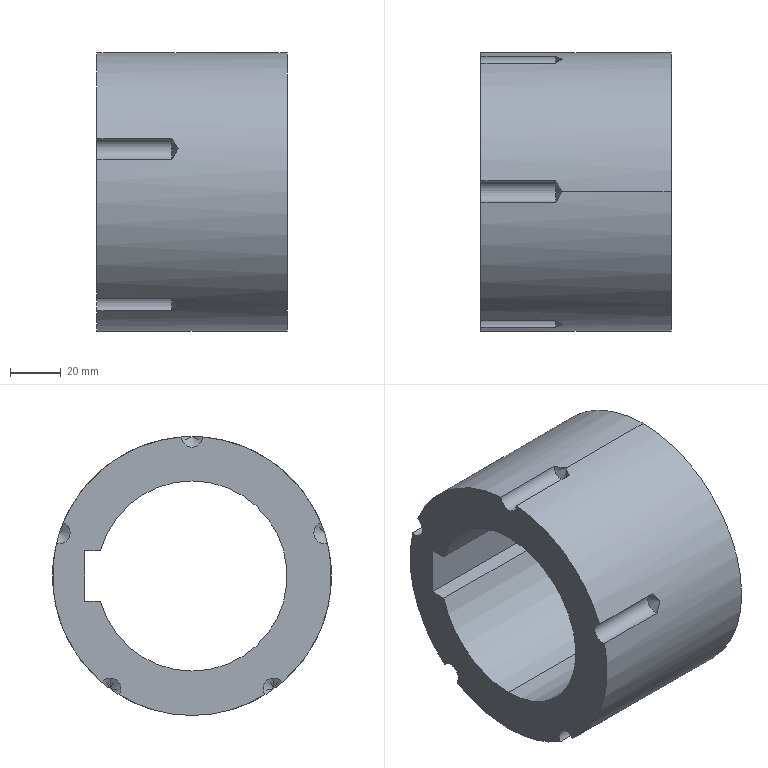Part | SolidWorks | features HoleWzd 1, ICE 1, Revolution 1 | 1 solid | 24 faces | box 75 x 110 x 110 mm | volume 369149 mm3 | cylinder 12 | cone 7 | plane 5 | commonest cylinder face diameters 8.5 x7 75 x3 110 x2
STEP:
#1=CARTESIAN_POINT('',(32.054,-32.328,-44.496));
#2=VERTEX_POINT('',#1);
#3=CARTESIAN_POINT('',(29.5,-28.796,-46.859));
#4=VERTEX_POINT('',#3);
#5=CARTESIAN_POINT('',(32.054,-32.328,-44.496));
#6=CARTESIAN_POINT('',(31.202,-31.182,-45.329));
#7=CARTESIAN_POINT('',(30.351,-30.003,-46.118));
#8=CARTESIAN_POINT('',(29.5,-28.796,-46.859));
#9=B_SPLINE_CURVE_WITH_KNOTS('',3,(#5,#6,#7,#8),.UNSPECIFIED.,.F.,.F.,(4,4),(-0.000000022,0.00496),.UNSPECIFIED.);
#10=EDGE_CURVE('',#2,#4,#9,.T.);
#11=ORIENTED_EDGE('',*,*,#10,.F.);
#12=CARTESIAN_POINT('',(29.5,-32.328,-40.246));
#13=VERTEX_POINT('',#12);
#14=CARTESIAN_POINT('',(29.5,-32.328,-40.246));
#15=DIRECTION('',(-0.515,0.,0.8572));
#16=VECTOR('',#15,1000.);
#17=LINE('',#14,#16);
#18=EDGE_CURVE('',#2,#13,#17,.T.);
#19=ORIENTED_EDGE('',*,*,#18,.T.);
#20=CARTESIAN_POINT('',(29.5,-32.328,-44.496));
#21=DIRECTION('',(-1.,0.,0.));
#22=DIRECTION('',(0.,0.,1.));
#23=AXIS2_PLACEMENT_3D('',#20,#21,#22);
#24=CIRCLE('',#23,4.25);
#25=EDGE_CURVE('',#13,#4,#24,.T.);
#26=ORIENTED_EDGE('',*,*,#25,.T.);
#27=EDGE_LOOP('',(#11,#19,#26));
#28=FACE_OUTER_BOUND('',#27,.T.);
#29=CARTESIAN_POINT('',(29.5,-32.328,-44.496));
#30=DIRECTION('',(-1.,0.,0.));
#31=DIRECTION('',(0.,0.,1.));
#32=AXIS2_PLACEMENT_3D('',#29,#30,#31);
#33=CONICAL_SURFACE('',#32,4.25,1.03);
#34=ADVANCED_FACE('',(#28),#33,.F.);
#35=ORIENTED_EDGE('',*,*,#25,.F.);
#36=CARTESIAN_POINT('',(0.,-32.328,-40.246));
#37=VERTEX_POINT('',#36);
#38=CARTESIAN_POINT('',(0.,-32.328,-40.246));
#39=DIRECTION('',(-1.,0.,0.));
#40=VECTOR('',#39,1000.);
#41=LINE('',#38,#40);
#42=EDGE_CURVE('',#13,#37,#41,.T.);
#43=ORIENTED_EDGE('',*,*,#42,.T.);
#44=CARTESIAN_POINT('',(0.,-28.796,-46.859));
#45=VERTEX_POINT('',#44);
#46=CARTESIAN_POINT('',(0.,-32.328,-44.496));
#47=DIRECTION('',(-1.,0.,0.));
#48=DIRECTION('',(0.,0.,1.));
#49=AXIS2_PLACEMENT_3D('',#46,#47,#48);
#50=CIRCLE('',#49,4.25);
#51=EDGE_CURVE('',#37,#45,#50,.T.);
#52=ORIENTED_EDGE('',*,*,#51,.T.);
#53=CARTESIAN_POINT('',(14.75,-28.796,-46.859));
#54=DIRECTION('',(-1.,0.,0.));
#55=VECTOR('',#54,1000.);
#56=LINE('',#53,#55);
#57=EDGE_CURVE('',#4,#45,#56,.T.);
#58=ORIENTED_EDGE('',*,*,#57,.F.);
#59=EDGE_LOOP('',(#35,#43,#52,#58));
#60=FACE_OUTER_BOUND('',#59,.T.);
#61=CARTESIAN_POINT('',(0.,-32.328,-44.496));
#62=DIRECTION('',(-1.,0.,0.));
#63=DIRECTION('',(0.,0.,1.));
#64=AXIS2_PLACEMENT_3D('',#61,#62,#63);
#65=CYLINDRICAL_SURFACE('',#64,4.25);
#66=ADVANCED_FACE('',(#60),#65,.F.);
#67=CARTESIAN_POINT('',(32.054,32.328,-44.496));
#68=VERTEX_POINT('',#67);
#69=CARTESIAN_POINT('',(29.5,35.667,-41.867));
#70=VERTEX_POINT('',#69);
#71=CARTESIAN_POINT('',(32.054,32.328,-44.496));
#72=CARTESIAN_POINT('',(31.202,33.475,-43.663));
#73=CARTESIAN_POINT('',(30.351,34.589,-42.785));
#74=CARTESIAN_POINT('',(29.5,35.667,-41.867));
#75=B_SPLINE_CURVE_WITH_KNOTS('',3,(#71,#72,#73,#74),.UNSPECIFIED.,.F.,.F.,(4,4),(-0.000000022,0.00496),.UNSPECIFIED.);
#76=EDGE_CURVE('',#68,#70,#75,.T.);
#77=ORIENTED_EDGE('',*,*,#76,.F.);
#78=CARTESIAN_POINT('',(29.5,32.328,-40.246));
#79=VERTEX_POINT('',#78);
#80=CARTESIAN_POINT('',(29.5,32.328,-40.246));
#81=DIRECTION('',(-0.515,0.,0.8572));
#82=VECTOR('',#81,1000.);
#83=LINE('',#80,#82);
#84=EDGE_CURVE('',#68,#79,#83,.T.);
#85=ORIENTED_EDGE('',*,*,#84,.T.);
#86=CARTESIAN_POINT('',(29.5,32.328,-44.496));
#87=DIRECTION('',(-1.,0.,0.));
#88=DIRECTION('',(0.,0.,1.));
#89=AXIS2_PLACEMENT_3D('',#86,#87,#88);
#90=CIRCLE('',#89,4.25);
#91=EDGE_CURVE('',#79,#70,#90,.T.);
#92=ORIENTED_EDGE('',*,*,#91,.T.);
#93=EDGE_LOOP('',(#77,#85,#92));
#94=FACE_OUTER_BOUND('',#93,.T.);
#95=CARTESIAN_POINT('',(29.5,32.328,-44.496));
#96=DIRECTION('',(-1.,0.,0.));
#97=DIRECTION('',(0.,0.,1.));
#98=AXIS2_PLACEMENT_3D('',#95,#96,#97);
#99=CONICAL_SURFACE('',#98,4.25,1.03);
#100=ADVANCED_FACE('',(#94),#99,.F.);
#101=ORIENTED_EDGE('',*,*,#91,.F.);
#102=CARTESIAN_POINT('',(0.,32.328,-40.246));
#103=VERTEX_POINT('',#102);
#104=CARTESIAN_POINT('',(0.,32.328,-40.246));
#105=DIRECTION('',(-1.,0.,0.));
#106=VECTOR('',#105,1000.);
#107=LINE('',#104,#106);
#108=EDGE_CURVE('',#79,#103,#107,.T.);
#109=ORIENTED_EDGE('',*,*,#108,.T.);
#110=CARTESIAN_POINT('',(0.,35.667,-41.867));
#111=VERTEX_POINT('',#110);
#112=CARTESIAN_POINT('',(0.,32.328,-44.496));
#113=DIRECTION('',(-1.,0.,0.));
#114=DIRECTION('',(0.,0.,1.));
#115=AXIS2_PLACEMENT_3D('',#112,#113,#114);
#116=CIRCLE('',#115,4.25);
#117=EDGE_CURVE('',#103,#111,#116,.T.);
#118=ORIENTED_EDGE('',*,*,#117,.T.);
#119=CARTESIAN_POINT('',(14.75,35.667,-41.867));
#120=DIRECTION('',(-1.,0.,0.));
#121=VECTOR('',#120,1000.);
#122=LINE('',#119,#121);
#123=EDGE_CURVE('',#70,#111,#122,.T.);
#124=ORIENTED_EDGE('',*,*,#123,.F.);
#125=EDGE_LOOP('',(#101,#109,#118,#124));
#126=FACE_OUTER_BOUND('',#125,.T.);
#127=CARTESIAN_POINT('',(0.,32.328,-44.496));
#128=DIRECTION('',(-1.,0.,0.));
#129=DIRECTION('',(0.,0.,1.));
#130=AXIS2_PLACEMENT_3D('',#127,#128,#129);
#131=CYLINDRICAL_SURFACE('',#130,4.25);
#132=ADVANCED_FACE('',(#126),#131,.F.);
#133=CARTESIAN_POINT('',(75.,0.,55.));
#134=VERTEX_POINT('',#133);
#135=CARTESIAN_POINT('',(75.,0.,-55.));
#136=VERTEX_POINT('',#135);
#137=CARTESIAN_POINT('',(75.,0.,0.));
#138=DIRECTION('',(-1.,0.,0.));
#139=DIRECTION('',(0.,0.,1.));
#140=AXIS2_PLACEMENT_3D('',#137,#138,#139);
#141=CIRCLE('',#140,55.);
#142=EDGE_CURVE('',#134,#136,#141,.T.);
#143=ORIENTED_EDGE('',*,*,#142,.T.);
#144=CARTESIAN_POINT('',(0.,0.,-55.));
#145=VERTEX_POINT('',#144);
#146=CARTESIAN_POINT('',(0.,0.,-55.));
#147=DIRECTION('',(-1.,0.,0.));
#148=VECTOR('',#147,1000.);
#149=LINE('',#146,#148);
#150=EDGE_CURVE('',#136,#145,#149,.T.);
#151=ORIENTED_EDGE('',*,*,#150,.T.);
#152=CARTESIAN_POINT('',(0.,28.796,-46.859));
#153=VERTEX_POINT('',#152);
#154=CARTESIAN_POINT('',(0.,0.,0.));
#155=DIRECTION('',(-1.,0.,0.));
#156=DIRECTION('',(0.,0.,1.));
#157=AXIS2_PLACEMENT_3D('',#154,#155,#156);
#158=CIRCLE('',#157,55.);
#159=EDGE_CURVE('',#153,#145,#158,.T.);
#160=ORIENTED_EDGE('',*,*,#159,.F.);
#161=CARTESIAN_POINT('',(29.5,28.796,-46.859));
#162=VERTEX_POINT('',#161);
#163=CARTESIAN_POINT('',(14.75,28.796,-46.859));
#164=DIRECTION('',(1.,0.,0.));
#165=VECTOR('',#164,1000.);
#166=LINE('',#163,#165);
#167=EDGE_CURVE('',#153,#162,#166,.T.);
#168=ORIENTED_EDGE('',*,*,#167,.T.);
#169=CARTESIAN_POINT('',(29.5,28.796,-46.859));
#170=CARTESIAN_POINT('',(29.925,29.399,-46.488));
#171=CARTESIAN_POINT('',(30.351,29.996,-46.106));
#172=CARTESIAN_POINT('',(30.989,30.879,-45.515));
#173=CARTESIAN_POINT('',(31.202,31.172,-45.315));
#174=CARTESIAN_POINT('',(31.628,31.753,-44.91));
#175=CARTESIAN_POINT('',(31.842,32.043,-44.703));
#176=CARTESIAN_POINT('',(32.054,32.328,-44.496));
#177=B_SPLINE_CURVE_WITH_KNOTS('',3,(#169,#170,#171,#172,#173,#174,#175,#176),.UNSPECIFIED.,.F.,.F.,(4,2,2,4),(0.01174,0.01422,0.01545,0.01669),.UNSPECIFIED.);
#178=EDGE_CURVE('',#162,#68,#177,.T.);
#179=ORIENTED_EDGE('',*,*,#178,.T.);
#180=ORIENTED_EDGE('',*,*,#76,.T.);
#181=ORIENTED_EDGE('',*,*,#123,.T.);
#182=CARTESIAN_POINT('',(0.,53.464,12.906));
#183=VERTEX_POINT('',#182);
#184=CARTESIAN_POINT('',(0.,0.,0.));
#185=DIRECTION('',(-1.,0.,0.));
#186=DIRECTION('',(0.,0.,1.));
#187=AXIS2_PLACEMENT_3D('',#184,#185,#186);
#188=CIRCLE('',#187,55.);
#189=EDGE_CURVE('',#183,#111,#188,.T.);
#190=ORIENTED_EDGE('',*,*,#189,.F.);
#191=CARTESIAN_POINT('',(29.5,53.464,12.906));
#192=VERTEX_POINT('',#191);
#193=CARTESIAN_POINT('',(14.75,53.464,12.906));
#194=DIRECTION('',(1.,0.,0.));
#195=VECTOR('',#194,1000.);
#196=LINE('',#193,#195);
#197=EDGE_CURVE('',#183,#192,#196,.T.);
#198=ORIENTED_EDGE('',*,*,#197,.T.);
#199=CARTESIAN_POINT('',(32.054,52.308,16.996));
#200=VERTEX_POINT('',#199);
#201=CARTESIAN_POINT('',(29.5,53.464,12.906));
#202=CARTESIAN_POINT('',(29.925,53.298,13.595));
#203=CARTESIAN_POINT('',(30.351,53.118,14.281));
#204=CARTESIAN_POINT('',(30.989,52.829,15.303));
#205=CARTESIAN_POINT('',(31.202,52.73,15.643));
#206=CARTESIAN_POINT('',(31.628,52.524,16.321));
#207=CARTESIAN_POINT('',(31.841,52.417,16.66));
#208=CARTESIAN_POINT('',(32.054,52.308,16.996));
#209=B_SPLINE_CURVE_WITH_KNOTS('',3,(#201,#202,#203,#204,#205,#206,#207,#208),.UNSPECIFIED.,.F.,.F.,(4,2,2,4),(0.01071,0.01319,0.01442,0.01566),.UNSPECIFIED.);
#210=EDGE_CURVE('',#192,#200,#209,.T.);
#211=ORIENTED_EDGE('',*,*,#210,.T.);
#212=CARTESIAN_POINT('',(29.5,50.84,20.984));
#213=VERTEX_POINT('',#212);
#214=CARTESIAN_POINT('',(32.054,52.308,16.996));
#215=CARTESIAN_POINT('',(31.202,51.87,18.344));
#216=CARTESIAN_POINT('',(30.351,51.38,19.675));
#217=CARTESIAN_POINT('',(29.5,50.84,20.984));
#218=B_SPLINE_CURVE_WITH_KNOTS('',3,(#214,#215,#216,#217),.UNSPECIFIED.,.F.,.F.,(4,4),(-0.000000022,0.00496),.UNSPECIFIED.);
#219=EDGE_CURVE('',#200,#213,#218,.T.);
#220=ORIENTED_EDGE('',*,*,#219,.T.);
#221=CARTESIAN_POINT('',(0.,50.84,20.984));
#222=VERTEX_POINT('',#221);
#223=CARTESIAN_POINT('',(14.75,50.84,20.984));
#224=DIRECTION('',(-1.,0.,0.));
#225=VECTOR('',#224,1000.);
#226=LINE('',#223,#225);
#227=EDGE_CURVE('',#213,#222,#226,.T.);
#228=ORIENTED_EDGE('',*,*,#227,.T.);
#229=CARTESIAN_POINT('',(0.,4.247,54.836));
#230=VERTEX_POINT('',#229);
#231=CARTESIAN_POINT('',(0.,0.,0.));
#232=DIRECTION('',(-1.,0.,0.));
#233=DIRECTION('',(0.,0.,1.));
#234=AXIS2_PLACEMENT_3D('',#231,#232,#233);
#235=CIRCLE('',#234,55.);
#236=EDGE_CURVE('',#230,#222,#235,.T.);
#237=ORIENTED_EDGE('',*,*,#236,.F.);
#238=CARTESIAN_POINT('',(29.5,4.247,54.836));
#239=VERTEX_POINT('',#238);
#240=CARTESIAN_POINT('',(14.75,4.247,54.836));
#241=DIRECTION('',(1.,0.,0.));
#242=VECTOR('',#241,1000.);
#243=LINE('',#240,#242);
#244=EDGE_CURVE('',#230,#239,#243,.T.);
#245=ORIENTED_EDGE('',*,*,#244,.T.);
#246=CARTESIAN_POINT('',(32.054,0.,55.));
#247=VERTEX_POINT('',#246);
#248=CARTESIAN_POINT('',(29.5,4.247,54.836));
#249=CARTESIAN_POINT('',(29.925,3.541,54.89));
#250=CARTESIAN_POINT('',(30.351,2.833,54.932));
#251=CARTESIAN_POINT('',(31.202,1.417,54.986));
#252=CARTESIAN_POINT('',(31.629,0.707,55.));
#253=CARTESIAN_POINT('',(32.054,0.,55.));
#254=B_SPLINE_CURVE_WITH_KNOTS('',3,(#248,#249,#250,#251,#252,#253),.UNSPECIFIED.,.F.,.F.,(4,2,4),(0.009274,0.01175,0.01422),.UNSPECIFIED.);
#255=EDGE_CURVE('',#239,#247,#254,.T.);
#256=ORIENTED_EDGE('',*,*,#255,.T.);
#257=CARTESIAN_POINT('',(0.,0.,55.));
#258=DIRECTION('',(-1.,0.,0.));
#259=VECTOR('',#258,1000.);
#260=LINE('',#257,#259);
#261=EDGE_CURVE('',#134,#247,#260,.T.);
#262=ORIENTED_EDGE('',*,*,#261,.F.);
#263=EDGE_LOOP('',(#143,#151,#160,#168,#179,#180,#181,#190,#198,#211,#220,#228,#237,#245,#256,#262));
#264=FACE_OUTER_BOUND('',#263,.T.);
#265=CARTESIAN_POINT('',(0.,0.,0.));
#266=DIRECTION('',(-1.,0.,0.));
#267=DIRECTION('',(0.,0.,1.));
#268=AXIS2_PLACEMENT_3D('',#265,#266,#267);
#269=CYLINDRICAL_SURFACE('',#268,55.);
#270=ADVANCED_FACE('',(#264),#269,.T.);
#271=CARTESIAN_POINT('',(75.,0.,-37.5));
#272=VERTEX_POINT('',#271);
#273=CARTESIAN_POINT('',(75.,0.,37.5));
#274=VERTEX_POINT('',#273);
#275=CARTESIAN_POINT('',(75.,0.,0.));
#276=DIRECTION('',(-1.,0.,0.));
#277=DIRECTION('',(0.,0.,1.));
#278=AXIS2_PLACEMENT_3D('',#275,#276,#277);
#279=CIRCLE('',#278,37.5);
#280=EDGE_CURVE('',#272,#274,#279,.T.);
#281=ORIENTED_EDGE('',*,*,#280,.F.);
#282=CARTESIAN_POINT('',(0.,0.,-37.5));
#283=VERTEX_POINT('',#282);
#284=CARTESIAN_POINT('',(0.,0.,-37.5));
#285=DIRECTION('',(-1.,0.,0.));
#286=VECTOR('',#285,1000.);
#287=LINE('',#284,#286);
#288=EDGE_CURVE('',#272,#283,#287,.T.);
#289=ORIENTED_EDGE('',*,*,#288,.T.);
#290=CARTESIAN_POINT('',(0.,0.,37.5));
#291=VERTEX_POINT('',#290);
#292=CARTESIAN_POINT('',(0.,0.,0.));
#293=DIRECTION('',(-1.,0.,0.));
#294=DIRECTION('',(0.,0.,1.));
#295=AXIS2_PLACEMENT_3D('',#292,#293,#294);
#296=CIRCLE('',#295,37.5);
#297=EDGE_CURVE('',#283,#291,#296,.T.);
#298=ORIENTED_EDGE('',*,*,#297,.T.);
#299=CARTESIAN_POINT('',(0.,0.,37.5));
#300=DIRECTION('',(-1.,0.,0.));
#301=VECTOR('',#300,1000.);
#302=LINE('',#299,#301);
#303=EDGE_CURVE('',#274,#291,#302,.T.);
#304=ORIENTED_EDGE('',*,*,#303,.F.);
#305=EDGE_LOOP('',(#281,#289,#298,#304));
#306=FACE_OUTER_BOUND('',#305,.T.);
#307=CARTESIAN_POINT('',(0.,0.,0.));
#308=DIRECTION('',(-1.,0.,0.));
#309=DIRECTION('',(0.,0.,1.));
#310=AXIS2_PLACEMENT_3D('',#307,#308,#309);
#311=CYLINDRICAL_SURFACE('',#310,37.5);
#312=ADVANCED_FACE('',(#306),#311,.F.);
#313=CARTESIAN_POINT('',(75.,36.142,10.));
#314=VERTEX_POINT('',#313);
#315=CARTESIAN_POINT('',(75.,0.,0.));
#316=DIRECTION('',(-1.,0.,0.));
#317=DIRECTION('',(0.,0.,1.));
#318=AXIS2_PLACEMENT_3D('',#315,#316,#317);
#319=CIRCLE('',#318,37.5);
#320=EDGE_CURVE('',#274,#314,#319,.T.);
#321=ORIENTED_EDGE('',*,*,#320,.F.);
#322=ORIENTED_EDGE('',*,*,#303,.T.);
#323=CARTESIAN_POINT('',(0.,36.142,10.));
#324=VERTEX_POINT('',#323);
#325=CARTESIAN_POINT('',(0.,0.,0.));
#326=DIRECTION('',(-1.,0.,0.));
#327=DIRECTION('',(0.,0.,1.));
#328=AXIS2_PLACEMENT_3D('',#325,#326,#327);
#329=CIRCLE('',#328,37.5);
#330=EDGE_CURVE('',#291,#324,#329,.T.);
#331=ORIENTED_EDGE('',*,*,#330,.T.);
#332=CARTESIAN_POINT('',(0.,36.142,10.));
#333=DIRECTION('',(-1.,0.,0.));
#334=VECTOR('',#333,1000.);
#335=LINE('',#332,#334);
#336=EDGE_CURVE('',#314,#324,#335,.T.);
#337=ORIENTED_EDGE('',*,*,#336,.F.);
#338=EDGE_LOOP('',(#321,#322,#331,#337));
#339=FACE_OUTER_BOUND('',#338,.T.);
#340=CARTESIAN_POINT('',(0.,0.,0.));
#341=DIRECTION('',(-1.,0.,0.));
#342=DIRECTION('',(0.,0.,1.));
#343=AXIS2_PLACEMENT_3D('',#340,#341,#342);
#344=CYLINDRICAL_SURFACE('',#343,37.5);
#345=ADVANCED_FACE('',(#339),#344,.F.);
#346=CARTESIAN_POINT('',(0.,36.142,-10.));
#347=VERTEX_POINT('',#346);
#348=CARTESIAN_POINT('',(0.,0.,0.));
#349=DIRECTION('',(-1.,0.,0.));
#350=DIRECTION('',(0.,0.,1.));
#351=AXIS2_PLACEMENT_3D('',#348,#349,#350);
#352=CIRCLE('',#351,37.5);
#353=EDGE_CURVE('',#347,#283,#352,.T.);
#354=ORIENTED_EDGE('',*,*,#353,.F.);
#355=CARTESIAN_POINT('',(0.,42.4,-10.));
#356=VERTEX_POINT('',#355);
#357=CARTESIAN_POINT('',(0.,-55.001,-10.));
#358=DIRECTION('',(0.,1.,0.));
#359=VECTOR('',#358,1000.);
#360=LINE('',#357,#359);
#361=EDGE_CURVE('',#347,#356,#360,.T.);
#362=ORIENTED_EDGE('',*,*,#361,.T.);
#363=CARTESIAN_POINT('',(0.,42.4,10.));
#364=VERTEX_POINT('',#363);
#365=CARTESIAN_POINT('',(0.,42.4,-10.));
#366=DIRECTION('',(0.,0.,1.));
#367=VECTOR('',#366,1000.);
#368=LINE('',#365,#367);
#369=EDGE_CURVE('',#356,#364,#368,.T.);
#370=ORIENTED_EDGE('',*,*,#369,.T.);
#371=CARTESIAN_POINT('',(0.,-55.001,10.));
#372=DIRECTION('',(0.,1.,0.));
#373=VECTOR('',#372,1000.);
#374=LINE('',#371,#373);
#375=EDGE_CURVE('',#324,#364,#374,.T.);
#376=ORIENTED_EDGE('',*,*,#375,.F.);
#377=ORIENTED_EDGE('',*,*,#330,.F.);
#378=ORIENTED_EDGE('',*,*,#297,.F.);
#379=EDGE_LOOP('',(#354,#362,#370,#376,#377,#378));
#380=FACE_BOUND('',#379,.T.);
#381=CARTESIAN_POINT('',(0.,-50.84,20.984));
#382=VERTEX_POINT('',#381);
#383=CARTESIAN_POINT('',(0.,-4.247,54.836));
#384=VERTEX_POINT('',#383);
#385=CARTESIAN_POINT('',(0.,0.,0.));
#386=DIRECTION('',(-1.,0.,0.));
#387=DIRECTION('',(0.,0.,1.));
#388=AXIS2_PLACEMENT_3D('',#385,#386,#387);
#389=CIRCLE('',#388,55.);
#390=EDGE_CURVE('',#382,#384,#389,.T.);
#391=ORIENTED_EDGE('',*,*,#390,.T.);
#392=CARTESIAN_POINT('',(0.,0.,55.));
#393=DIRECTION('',(-1.,0.,0.));
#394=DIRECTION('',(0.,0.,1.));
#395=AXIS2_PLACEMENT_3D('',#392,#393,#394);
#396=CIRCLE('',#395,4.25);
#397=EDGE_CURVE('',#230,#384,#396,.T.);
#398=ORIENTED_EDGE('',*,*,#397,.F.);
#399=ORIENTED_EDGE('',*,*,#236,.T.);
#400=CARTESIAN_POINT('',(0.,52.308,16.996));
#401=DIRECTION('',(-1.,0.,0.));
#402=DIRECTION('',(0.,0.,1.));
#403=AXIS2_PLACEMENT_3D('',#400,#401,#402);
#404=CIRCLE('',#403,4.25);
#405=EDGE_CURVE('',#183,#222,#404,.T.);
#406=ORIENTED_EDGE('',*,*,#405,.F.);
#407=ORIENTED_EDGE('',*,*,#189,.T.);
#408=ORIENTED_EDGE('',*,*,#117,.F.);
#409=CARTESIAN_POINT('',(0.,32.328,-44.496));
#410=DIRECTION('',(-1.,0.,0.));
#411=DIRECTION('',(0.,0.,1.));
#412=AXIS2_PLACEMENT_3D('',#409,#410,#411);
#413=CIRCLE('',#412,4.25);
#414=EDGE_CURVE('',#153,#103,#413,.T.);
#415=ORIENTED_EDGE('',*,*,#414,.F.);
#416=ORIENTED_EDGE('',*,*,#159,.T.);
#417=CARTESIAN_POINT('',(0.,0.,0.));
#418=DIRECTION('',(-1.,0.,0.));
#419=DIRECTION('',(0.,0.,1.));
#420=AXIS2_PLACEMENT_3D('',#417,#418,#419);
#421=CIRCLE('',#420,55.);
#422=EDGE_CURVE('',#145,#45,#421,.T.);
#423=ORIENTED_EDGE('',*,*,#422,.T.);
#424=ORIENTED_EDGE('',*,*,#51,.F.);
#425=CARTESIAN_POINT('',(0.,-35.667,-41.867));
#426=VERTEX_POINT('',#425);
#427=CARTESIAN_POINT('',(0.,-32.328,-44.496));
#428=DIRECTION('',(-1.,0.,0.));
#429=DIRECTION('',(0.,0.,1.));
#430=AXIS2_PLACEMENT_3D('',#427,#428,#429);
#431=CIRCLE('',#430,4.25);
#432=EDGE_CURVE('',#426,#37,#431,.T.);
#433=ORIENTED_EDGE('',*,*,#432,.F.);
#434=CARTESIAN_POINT('',(0.,-53.464,12.906));
#435=VERTEX_POINT('',#434);
#436=CARTESIAN_POINT('',(0.,0.,0.));
#437=DIRECTION('',(-1.,0.,0.));
#438=DIRECTION('',(0.,0.,1.));
#439=AXIS2_PLACEMENT_3D('',#436,#437,#438);
#440=CIRCLE('',#439,55.);
#441=EDGE_CURVE('',#426,#435,#440,.T.);
#442=ORIENTED_EDGE('',*,*,#441,.T.);
#443=CARTESIAN_POINT('',(0.,-52.308,16.996));
#444=DIRECTION('',(-1.,0.,0.));
#445=DIRECTION('',(0.,0.,1.));
#446=AXIS2_PLACEMENT_3D('',#443,#444,#445);
#447=CIRCLE('',#446,4.25);
#448=EDGE_CURVE('',#382,#435,#447,.T.);
#449=ORIENTED_EDGE('',*,*,#448,.F.);
#450=EDGE_LOOP('',(#391,#398,#399,#406,#407,#408,#415,#416,#423,#424,#433,#442,#449));
#451=FACE_OUTER_BOUND('',#450,.T.);
#452=CARTESIAN_POINT('',(0.,55.,0.));
#453=DIRECTION('',(1.,0.,0.));
#454=DIRECTION('',(0.,0.,-1.));
#455=AXIS2_PLACEMENT_3D('',#452,#453,#454);
#456=PLANE('',#455);
#457=ADVANCED_FACE('',(#380,#451),#456,.F.);
#458=ORIENTED_EDGE('',*,*,#288,.F.);
#459=CARTESIAN_POINT('',(75.,36.142,-10.));
#460=VERTEX_POINT('',#459);
#461=CARTESIAN_POINT('',(75.,0.,0.));
#462=DIRECTION('',(-1.,0.,0.));
#463=DIRECTION('',(0.,0.,1.));
#464=AXIS2_PLACEMENT_3D('',#461,#462,#463);
#465=CIRCLE('',#464,37.5);
#466=EDGE_CURVE('',#460,#272,#465,.T.);
#467=ORIENTED_EDGE('',*,*,#466,.F.);
#468=CARTESIAN_POINT('',(0.,36.142,-10.));
#469=DIRECTION('',(1.,0.,0.));
#470=VECTOR('',#469,1000.);
#471=LINE('',#468,#470);
#472=EDGE_CURVE('',#347,#460,#471,.T.);
#473=ORIENTED_EDGE('',*,*,#472,.F.);
#474=ORIENTED_EDGE('',*,*,#353,.T.);
#475=EDGE_LOOP('',(#458,#467,#473,#474));
#476=FACE_OUTER_BOUND('',#475,.T.);
#477=CARTESIAN_POINT('',(0.,0.,0.));
#478=DIRECTION('',(-1.,0.,0.));
#479=DIRECTION('',(0.,0.,1.));
#480=AXIS2_PLACEMENT_3D('',#477,#478,#479);
#481=CYLINDRICAL_SURFACE('',#480,37.5);
#482=ADVANCED_FACE('',(#476),#481,.F.);
#483=ORIENTED_EDGE('',*,*,#142,.F.);
#484=CARTESIAN_POINT('',(75.,0.,0.));
#485=DIRECTION('',(-1.,0.,0.));
#486=DIRECTION('',(0.,0.,1.));
#487=AXIS2_PLACEMENT_3D('',#484,#485,#486);
#488=CIRCLE('',#487,55.);
#489=EDGE_CURVE('',#136,#134,#488,.T.);
#490=ORIENTED_EDGE('',*,*,#489,.F.);
#491=EDGE_LOOP('',(#483,#490));
#492=FACE_OUTER_BOUND('',#491,.T.);
#493=CARTESIAN_POINT('',(75.,42.4,10.));
#494=VERTEX_POINT('',#493);
#495=CARTESIAN_POINT('',(75.,42.4,-10.));
#496=VERTEX_POINT('',#495);
#497=CARTESIAN_POINT('',(75.,42.4,-10.));
#498=DIRECTION('',(0.,0.,-1.));
#499=VECTOR('',#498,1000.);
#500=LINE('',#497,#499);
#501=EDGE_CURVE('',#494,#496,#500,.T.);
#502=ORIENTED_EDGE('',*,*,#501,.T.);
#503=CARTESIAN_POINT('',(75.,-55.001,-10.));
#504=DIRECTION('',(0.,1.,0.));
#505=VECTOR('',#504,1000.);
#506=LINE('',#503,#505);
#507=EDGE_CURVE('',#460,#496,#506,.T.);
#508=ORIENTED_EDGE('',*,*,#507,.F.);
#509=ORIENTED_EDGE('',*,*,#466,.T.);
#510=ORIENTED_EDGE('',*,*,#280,.T.);
#511=ORIENTED_EDGE('',*,*,#320,.T.);
#512=CARTESIAN_POINT('',(75.,-55.001,10.));
#513=DIRECTION('',(0.,1.,0.));
#514=VECTOR('',#513,1000.);
#515=LINE('',#512,#514);
#516=EDGE_CURVE('',#314,#494,#515,.T.);
#517=ORIENTED_EDGE('',*,*,#516,.T.);
#518=EDGE_LOOP('',(#502,#508,#509,#510,#511,#517));
#519=FACE_BOUND('',#518,.T.);
#520=CARTESIAN_POINT('',(75.,55.,0.));
#521=DIRECTION('',(-1.,0.,0.));
#522=DIRECTION('',(0.,0.,1.));
#523=AXIS2_PLACEMENT_3D('',#520,#521,#522);
#524=PLANE('',#523);
#525=ADVANCED_FACE('',(#492,#519),#524,.F.);
#526=ORIENTED_EDGE('',*,*,#150,.F.);
#527=ORIENTED_EDGE('',*,*,#489,.T.);
#528=ORIENTED_EDGE('',*,*,#261,.T.);
#529=CARTESIAN_POINT('',(29.5,-4.247,54.836));
#530=VERTEX_POINT('',#529);
#531=CARTESIAN_POINT('',(32.054,0.,55.));
#532=CARTESIAN_POINT('',(31.202,-1.417,55.));
#533=CARTESIAN_POINT('',(30.351,-2.834,54.945));
#534=CARTESIAN_POINT('',(29.5,-4.247,54.836));
#535=B_SPLINE_CURVE_WITH_KNOTS('',3,(#531,#532,#533,#534),.UNSPECIFIED.,.F.,.F.,(4,4),(-0.000000022,0.00496),.UNSPECIFIED.);
#536=EDGE_CURVE('',#247,#530,#535,.T.);
#537=ORIENTED_EDGE('',*,*,#536,.T.);
#538=CARTESIAN_POINT('',(14.75,-4.247,54.836));
#539=DIRECTION('',(-1.,0.,0.));
#540=VECTOR('',#539,1000.);
#541=LINE('',#538,#540);
#542=EDGE_CURVE('',#530,#384,#541,.T.);
#543=ORIENTED_EDGE('',*,*,#542,.T.);
#544=ORIENTED_EDGE('',*,*,#390,.F.);
#545=CARTESIAN_POINT('',(29.5,-50.84,20.984));
#546=VERTEX_POINT('',#545);
#547=CARTESIAN_POINT('',(14.75,-50.84,20.984));
#548=DIRECTION('',(1.,0.,0.));
#549=VECTOR('',#548,1000.);
#550=LINE('',#547,#549);
#551=EDGE_CURVE('',#382,#546,#550,.T.);
#552=ORIENTED_EDGE('',*,*,#551,.T.);
#553=CARTESIAN_POINT('',(32.054,-52.308,16.996));
#554=VERTEX_POINT('',#553);
#555=CARTESIAN_POINT('',(29.5,-50.84,20.984));
#556=CARTESIAN_POINT('',(29.925,-51.11,20.329));
#557=CARTESIAN_POINT('',(30.351,-51.368,19.669));
#558=CARTESIAN_POINT('',(30.989,-51.735,18.672));
#559=CARTESIAN_POINT('',(31.202,-51.854,18.338));
#560=CARTESIAN_POINT('',(31.628,-52.086,17.669));
#561=CARTESIAN_POINT('',(31.841,-52.199,17.332));
#562=CARTESIAN_POINT('',(32.054,-52.308,16.996));
#563=B_SPLINE_CURVE_WITH_KNOTS('',3,(#555,#556,#557,#558,#559,#560,#561,#562),.UNSPECIFIED.,.F.,.F.,(4,2,2,4),(0.01071,0.01319,0.01442,0.01566),.UNSPECIFIED.);
#564=EDGE_CURVE('',#546,#554,#563,.T.);
#565=ORIENTED_EDGE('',*,*,#564,.T.);
#566=CARTESIAN_POINT('',(29.5,-53.464,12.906));
#567=VERTEX_POINT('',#566);
#568=CARTESIAN_POINT('',(32.054,-52.308,16.996));
#569=CARTESIAN_POINT('',(31.202,-52.746,15.648));
#570=CARTESIAN_POINT('',(30.351,-53.132,14.283));
#571=CARTESIAN_POINT('',(29.5,-53.464,12.906));
#572=B_SPLINE_CURVE_WITH_KNOTS('',3,(#568,#569,#570,#571),.UNSPECIFIED.,.F.,.F.,(4,4),(-0.000000022,0.00496),.UNSPECIFIED.);
#573=EDGE_CURVE('',#554,#567,#572,.T.);
#574=ORIENTED_EDGE('',*,*,#573,.T.);
#575=CARTESIAN_POINT('',(14.75,-53.464,12.906));
#576=DIRECTION('',(-1.,0.,0.));
#577=VECTOR('',#576,1000.);
#578=LINE('',#575,#577);
#579=EDGE_CURVE('',#567,#435,#578,.T.);
#580=ORIENTED_EDGE('',*,*,#579,.T.);
#581=ORIENTED_EDGE('',*,*,#441,.F.);
#582=CARTESIAN_POINT('',(29.5,-35.667,-41.867));
#583=VERTEX_POINT('',#582);
#584=CARTESIAN_POINT('',(14.75,-35.667,-41.867));
#585=DIRECTION('',(1.,0.,0.));
#586=VECTOR('',#585,1000.);
#587=LINE('',#584,#586);
#588=EDGE_CURVE('',#426,#583,#587,.T.);
#589=ORIENTED_EDGE('',*,*,#588,.T.);
#590=CARTESIAN_POINT('',(29.5,-35.667,-41.867));
#591=CARTESIAN_POINT('',(29.925,-35.128,-42.326));
#592=CARTESIAN_POINT('',(30.351,-34.58,-42.775));
#593=CARTESIAN_POINT('',(30.989,-33.745,-43.433));
#594=CARTESIAN_POINT('',(31.202,-33.464,-43.649));
#595=CARTESIAN_POINT('',(31.628,-32.899,-44.077));
#596=CARTESIAN_POINT('',(31.842,-32.614,-44.288));
#597=CARTESIAN_POINT('',(32.054,-32.328,-44.496));
#598=B_SPLINE_CURVE_WITH_KNOTS('',3,(#590,#591,#592,#593,#594,#595,#596,#597),.UNSPECIFIED.,.F.,.F.,(4,2,2,4),(0.01174,0.01422,0.01545,0.01669),.UNSPECIFIED.);
#599=EDGE_CURVE('',#583,#2,#598,.T.);
#600=ORIENTED_EDGE('',*,*,#599,.T.);
#601=ORIENTED_EDGE('',*,*,#10,.T.);
#602=ORIENTED_EDGE('',*,*,#57,.T.);
#603=ORIENTED_EDGE('',*,*,#422,.F.);
#604=EDGE_LOOP('',(#526,#527,#528,#537,#543,#544,#552,#565,#574,#580,#581,#589,#600,#601,#602,#603));
#605=FACE_OUTER_BOUND('',#604,.T.);
#606=CARTESIAN_POINT('',(0.,0.,0.));
#607=DIRECTION('',(-1.,0.,0.));
#608=DIRECTION('',(0.,0.,1.));
#609=AXIS2_PLACEMENT_3D('',#606,#607,#608);
#610=CYLINDRICAL_SURFACE('',#609,55.);
#611=ADVANCED_FACE('',(#605),#610,.T.);
#612=ORIENTED_EDGE('',*,*,#472,.T.);
#613=ORIENTED_EDGE('',*,*,#507,.T.);
#614=CARTESIAN_POINT('',(0.,42.4,-10.));
#615=DIRECTION('',(-1.,0.,0.));
#616=VECTOR('',#615,1000.);
#617=LINE('',#614,#616);
#618=EDGE_CURVE('',#496,#356,#617,.T.);
#619=ORIENTED_EDGE('',*,*,#618,.T.);
#620=ORIENTED_EDGE('',*,*,#361,.F.);
#621=EDGE_LOOP('',(#612,#613,#619,#620));
#622=FACE_OUTER_BOUND('',#621,.T.);
#623=CARTESIAN_POINT('',(0.,-55.001,-10.));
#624=DIRECTION('',(0.,0.,-1.));
#625=DIRECTION('',(-1.,0.,0.));
#626=AXIS2_PLACEMENT_3D('',#623,#624,#625);
#627=PLANE('',#626);
#628=ADVANCED_FACE('',(#622),#627,.F.);
#629=ORIENTED_EDGE('',*,*,#336,.T.);
#630=ORIENTED_EDGE('',*,*,#375,.T.);
#631=CARTESIAN_POINT('',(0.,42.4,10.));
#632=DIRECTION('',(1.,0.,0.));
#633=VECTOR('',#632,1000.);
#634=LINE('',#631,#633);
#635=EDGE_CURVE('',#364,#494,#634,.T.);
#636=ORIENTED_EDGE('',*,*,#635,.T.);
#637=ORIENTED_EDGE('',*,*,#516,.F.);
#638=EDGE_LOOP('',(#629,#630,#636,#637));
#639=FACE_OUTER_BOUND('',#638,.T.);
#640=CARTESIAN_POINT('',(0.,-55.001,10.));
#641=DIRECTION('',(0.,0.,1.));
#642=DIRECTION('',(1.,0.,0.));
#643=AXIS2_PLACEMENT_3D('',#640,#641,#642);
#644=PLANE('',#643);
#645=ADVANCED_FACE('',(#639),#644,.F.);
#646=ORIENTED_EDGE('',*,*,#369,.F.);
#647=ORIENTED_EDGE('',*,*,#618,.F.);
#648=ORIENTED_EDGE('',*,*,#501,.F.);
#649=ORIENTED_EDGE('',*,*,#635,.F.);
#650=EDGE_LOOP('',(#646,#647,#648,#649));
#651=FACE_OUTER_BOUND('',#650,.T.);
#652=CARTESIAN_POINT('',(0.,42.4,0.));
#653=DIRECTION('',(0.,1.,0.));
#654=DIRECTION('',(0.,0.,1.));
#655=AXIS2_PLACEMENT_3D('',#652,#653,#654);
#656=PLANE('',#655);
#657=ADVANCED_FACE('',(#651),#656,.F.);
#658=ORIENTED_EDGE('',*,*,#405,.T.);
#659=ORIENTED_EDGE('',*,*,#227,.F.);
#660=CARTESIAN_POINT('',(29.5,52.308,16.996));
#661=DIRECTION('',(-1.,0.,0.));
#662=DIRECTION('',(0.,0.,1.));
#663=AXIS2_PLACEMENT_3D('',#660,#661,#662);
#664=CIRCLE('',#663,4.25);
#665=EDGE_CURVE('',#192,#213,#664,.T.);
#666=ORIENTED_EDGE('',*,*,#665,.F.);
#667=ORIENTED_EDGE('',*,*,#197,.F.);
#668=EDGE_LOOP('',(#658,#659,#666,#667));
#669=FACE_OUTER_BOUND('',#668,.T.);
#670=CARTESIAN_POINT('',(0.,52.308,16.996));
#671=DIRECTION('',(-1.,0.,0.));
#672=DIRECTION('',(0.,0.,1.));
#673=AXIS2_PLACEMENT_3D('',#670,#671,#672);
#674=CYLINDRICAL_SURFACE('',#673,4.25);
#675=ADVANCED_FACE('',(#669),#674,.F.);
#676=ORIENTED_EDGE('',*,*,#210,.F.);
#677=ORIENTED_EDGE('',*,*,#665,.T.);
#678=ORIENTED_EDGE('',*,*,#219,.F.);
#679=EDGE_LOOP('',(#676,#677,#678));
#680=FACE_OUTER_BOUND('',#679,.T.);
#681=CARTESIAN_POINT('',(29.5,52.308,16.996));
#682=DIRECTION('',(-1.,0.,0.));
#683=DIRECTION('',(0.,0.,1.));
#684=AXIS2_PLACEMENT_3D('',#681,#682,#683);
#685=CONICAL_SURFACE('',#684,4.25,1.03);
#686=ADVANCED_FACE('',(#680),#685,.F.);
#687=ORIENTED_EDGE('',*,*,#108,.F.);
#688=CARTESIAN_POINT('',(29.5,32.328,-44.496));
#689=DIRECTION('',(-1.,0.,0.));
#690=DIRECTION('',(0.,0.,1.));
#691=AXIS2_PLACEMENT_3D('',#688,#689,#690);
#692=CIRCLE('',#691,4.25);
#693=EDGE_CURVE('',#162,#79,#692,.T.);
#694=ORIENTED_EDGE('',*,*,#693,.F.);
#695=ORIENTED_EDGE('',*,*,#167,.F.);
#696=ORIENTED_EDGE('',*,*,#414,.T.);
#697=EDGE_LOOP('',(#687,#694,#695,#696));
#698=FACE_OUTER_BOUND('',#697,.T.);
#699=CARTESIAN_POINT('',(0.,32.328,-44.496));
#700=DIRECTION('',(-1.,0.,0.));
#701=DIRECTION('',(0.,0.,1.));
#702=AXIS2_PLACEMENT_3D('',#699,#700,#701);
#703=CYLINDRICAL_SURFACE('',#702,4.25);
#704=ADVANCED_FACE('',(#698),#703,.F.);
#705=ORIENTED_EDGE('',*,*,#84,.F.);
#706=ORIENTED_EDGE('',*,*,#178,.F.);
#707=ORIENTED_EDGE('',*,*,#693,.T.);
#708=EDGE_LOOP('',(#705,#706,#707));
#709=FACE_OUTER_BOUND('',#708,.T.);
#710=CARTESIAN_POINT('',(29.5,32.328,-44.496));
#711=DIRECTION('',(-1.,0.,0.));
#712=DIRECTION('',(0.,0.,1.));
#713=AXIS2_PLACEMENT_3D('',#710,#711,#712);
#714=CONICAL_SURFACE('',#713,4.25,1.03);
#715=ADVANCED_FACE('',(#709),#714,.F.);
#716=ORIENTED_EDGE('',*,*,#42,.F.);
#717=CARTESIAN_POINT('',(29.5,-32.328,-44.496));
#718=DIRECTION('',(-1.,0.,0.));
#719=DIRECTION('',(0.,0.,1.));
#720=AXIS2_PLACEMENT_3D('',#717,#718,#719);
#721=CIRCLE('',#720,4.25);
#722=EDGE_CURVE('',#583,#13,#721,.T.);
#723=ORIENTED_EDGE('',*,*,#722,.F.);
#724=ORIENTED_EDGE('',*,*,#588,.F.);
#725=ORIENTED_EDGE('',*,*,#432,.T.);
#726=EDGE_LOOP('',(#716,#723,#724,#725));
#727=FACE_OUTER_BOUND('',#726,.T.);
#728=CARTESIAN_POINT('',(0.,-32.328,-44.496));
#729=DIRECTION('',(-1.,0.,0.));
#730=DIRECTION('',(0.,0.,1.));
#731=AXIS2_PLACEMENT_3D('',#728,#729,#730);
#732=CYLINDRICAL_SURFACE('',#731,4.25);
#733=ADVANCED_FACE('',(#727),#732,.F.);
#734=ORIENTED_EDGE('',*,*,#18,.F.);
#735=ORIENTED_EDGE('',*,*,#599,.F.);
#736=ORIENTED_EDGE('',*,*,#722,.T.);
#737=EDGE_LOOP('',(#734,#735,#736));
#738=FACE_OUTER_BOUND('',#737,.T.);
#739=CARTESIAN_POINT('',(29.5,-32.328,-44.496));
#740=DIRECTION('',(-1.,0.,0.));
#741=DIRECTION('',(0.,0.,1.));
#742=AXIS2_PLACEMENT_3D('',#739,#740,#741);
#743=CONICAL_SURFACE('',#742,4.25,1.03);
#744=ADVANCED_FACE('',(#738),#743,.F.);
#745=ORIENTED_EDGE('',*,*,#448,.T.);
#746=ORIENTED_EDGE('',*,*,#579,.F.);
#747=CARTESIAN_POINT('',(29.5,-52.308,16.996));
#748=DIRECTION('',(-1.,0.,0.));
#749=DIRECTION('',(0.,0.,1.));
#750=AXIS2_PLACEMENT_3D('',#747,#748,#749);
#751=CIRCLE('',#750,4.25);
#752=EDGE_CURVE('',#546,#567,#751,.T.);
#753=ORIENTED_EDGE('',*,*,#752,.F.);
#754=ORIENTED_EDGE('',*,*,#551,.F.);
#755=EDGE_LOOP('',(#745,#746,#753,#754));
#756=FACE_OUTER_BOUND('',#755,.T.);
#757=CARTESIAN_POINT('',(0.,-52.308,16.996));
#758=DIRECTION('',(-1.,0.,0.));
#759=DIRECTION('',(0.,0.,1.));
#760=AXIS2_PLACEMENT_3D('',#757,#758,#759);
#761=CYLINDRICAL_SURFACE('',#760,4.25);
#762=ADVANCED_FACE('',(#756),#761,.F.);
#763=ORIENTED_EDGE('',*,*,#564,.F.);
#764=ORIENTED_EDGE('',*,*,#752,.T.);
#765=ORIENTED_EDGE('',*,*,#573,.F.);
#766=EDGE_LOOP('',(#763,#764,#765));
#767=FACE_OUTER_BOUND('',#766,.T.);
#768=CARTESIAN_POINT('',(29.5,-52.308,16.996));
#769=DIRECTION('',(-1.,0.,0.));
#770=DIRECTION('',(0.,0.,1.));
#771=AXIS2_PLACEMENT_3D('',#768,#769,#770);
#772=CONICAL_SURFACE('',#771,4.25,1.03);
#773=ADVANCED_FACE('',(#767),#772,.F.);
#774=ORIENTED_EDGE('',*,*,#397,.T.);
#775=ORIENTED_EDGE('',*,*,#542,.F.);
#776=CARTESIAN_POINT('',(29.5,0.,55.));
#777=DIRECTION('',(-1.,0.,0.));
#778=DIRECTION('',(0.,0.,1.));
#779=AXIS2_PLACEMENT_3D('',#776,#777,#778);
#780=CIRCLE('',#779,4.25);
#781=EDGE_CURVE('',#239,#530,#780,.T.);
#782=ORIENTED_EDGE('',*,*,#781,.F.);
#783=ORIENTED_EDGE('',*,*,#244,.F.);
#784=EDGE_LOOP('',(#774,#775,#782,#783));
#785=FACE_OUTER_BOUND('',#784,.T.);
#786=CARTESIAN_POINT('',(0.,0.,55.));
#787=DIRECTION('',(-1.,0.,0.));
#788=DIRECTION('',(0.,0.,1.));
#789=AXIS2_PLACEMENT_3D('',#786,#787,#788);
#790=CYLINDRICAL_SURFACE('',#789,4.25);
#791=ADVANCED_FACE('',(#785),#790,.F.);
#792=ORIENTED_EDGE('',*,*,#255,.F.);
#793=ORIENTED_EDGE('',*,*,#781,.T.);
#794=ORIENTED_EDGE('',*,*,#536,.F.);
#795=EDGE_LOOP('',(#792,#793,#794));
#796=FACE_OUTER_BOUND('',#795,.T.);
#797=CARTESIAN_POINT('',(29.5,0.,55.));
#798=DIRECTION('',(-1.,0.,0.));
#799=DIRECTION('',(0.,0.,1.));
#800=AXIS2_PLACEMENT_3D('',#797,#798,#799);
#801=CONICAL_SURFACE('',#800,4.25,1.03);
#802=ADVANCED_FACE('',(#796),#801,.F.);
#803=CLOSED_SHELL('',(#34,#66,#100,#132,#270,#312,#345,#457,#482,#525,#611,#628,#645,#657,#675,#686,#704,#715,#733,#744,#762,#773,#791,#802));
#804=MANIFOLD_SOLID_BREP('',#803);
#805=CARTESIAN_POINT('',(0.,0.,0.));
#806=DIRECTION('',(0.,0.,1.));
#807=DIRECTION('',(1.,0.,0.));
#808=AXIS2_PLACEMENT_3D('',#805,#806,#807);
#809=(LENGTH_UNIT()NAMED_UNIT(*)SI_UNIT(.MILLI.,.METRE.));
#810=UNCERTAINTY_MEASURE_WITH_UNIT(LENGTH_MEASURE(0.00001),#809,'','');
#811=(NAMED_UNIT(*)PLANE_ANGLE_UNIT()SI_UNIT($,.RADIAN.));
#812=(NAMED_UNIT(*)SI_UNIT($,.STERADIAN.)SOLID_ANGLE_UNIT());
#813=(GEOMETRIC_REPRESENTATION_CONTEXT(3)GLOBAL_UNCERTAINTY_ASSIGNED_CONTEXT((#810))GLOBAL_UNIT_ASSIGNED_CONTEXT((#809,#811,#812))REPRESENTATION_CONTEXT('',''));
#814=ADVANCED_BREP_SHAPE_REPRESENTATION('',(#804,#808),#813);